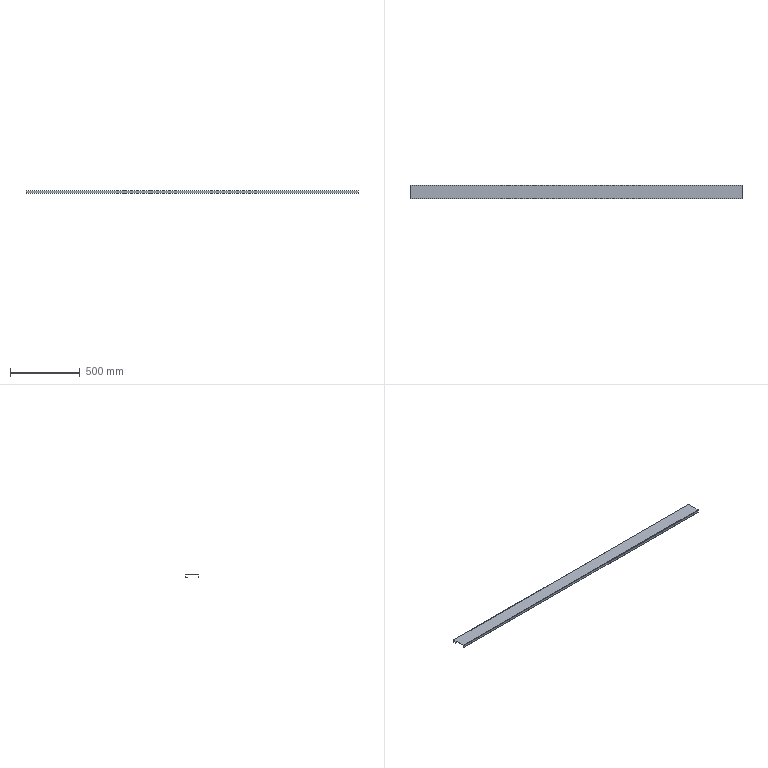Part | STEP file | E3-中转釜护栏4踢脚Plate | 1 solid | 18 faces | box 2388 x 100 x 20 mm | volume 548930 mm3 | plane 12 | cylinder 6 | commonest cylinder face diameters 2 x3 5 x3
STEP:
#1=CARTESIAN_POINT('',(0.,0.,0.));
#2=DIRECTION('',(0.,0.,1.));
#3=DIRECTION('',(1.,0.,0.));
#4=AXIS2_PLACEMENT_3D('',#1,#2,#3);
#5=CARTESIAN_POINT('',(-1194.,1.5,-2.5));
#6=VERTEX_POINT('',#5);
#7=CARTESIAN_POINT('',(-1194.,1.5,-20.));
#8=VERTEX_POINT('',#7);
#9=CARTESIAN_POINT('',(-1194.,1.5,-2.5));
#10=DIRECTION('',(0.,0.,-1.));
#11=VECTOR('',#10,1.);
#12=LINE('',#9,#11);
#13=CARTESIAN_POINT('',(1194.,1.5,-2.5));
#14=DIRECTION('',(0.,-1.,0.));
#15=DIRECTION('',(0.,0.,1.));
#16=AXIS2_PLACEMENT_3D('',#13,#14,#15);
#17=PLANE('',#16);
#18=CARTESIAN_POINT('',(0.,2388.));
#19=DIRECTION('',(-1.,0.));
#20=VECTOR('',#19,1.);
#21=LINE('',#18,#20);
#22=(GEOMETRIC_REPRESENTATION_CONTEXT(2)PARAMETRIC_REPRESENTATION_CONTEXT()REPRESENTATION_CONTEXT('',''));
#23=DEFINITIONAL_REPRESENTATION('',(#21),#22);
#24=PCURVE('',#17,#23);
#25=CARTESIAN_POINT('',(-1194.,2.5,-2.5));
#26=DIRECTION('',(-1.,0.,0.));
#27=DIRECTION('',(0.,0.,-1.));
#28=AXIS2_PLACEMENT_3D('',#25,#26,#27);
#29=PLANE('',#28);
#30=CARTESIAN_POINT('',(0.,1.));
#31=DIRECTION('',(1.,0.));
#32=VECTOR('',#31,1.);
#33=LINE('',#30,#32);
#34=(GEOMETRIC_REPRESENTATION_CONTEXT(2)PARAMETRIC_REPRESENTATION_CONTEXT()REPRESENTATION_CONTEXT('',''));
#35=DEFINITIONAL_REPRESENTATION('',(#33),#34);
#36=PCURVE('',#29,#35);
#37=SURFACE_CURVE('',#12,(#24,#36),.PCURVE_S1.);
#38=EDGE_CURVE('',#6,#8,#37,.T.);
#39=ORIENTED_EDGE('',*,*,#38,.F.);
#40=CARTESIAN_POINT('',(1194.,1.5,-2.5));
#41=VERTEX_POINT('',#40);
#42=CARTESIAN_POINT('',(1194.,1.5,-2.5));
#43=DIRECTION('',(-1.,0.,0.));
#44=VECTOR('',#43,1.);
#45=LINE('',#42,#44);
#46=CARTESIAN_POINT('',(0.,0.));
#47=DIRECTION('',(0.,1.));
#48=VECTOR('',#47,1.);
#49=LINE('',#46,#48);
#50=(GEOMETRIC_REPRESENTATION_CONTEXT(2)PARAMETRIC_REPRESENTATION_CONTEXT()REPRESENTATION_CONTEXT('',''));
#51=DEFINITIONAL_REPRESENTATION('',(#49),#50);
#52=PCURVE('',#17,#51);
#53=CARTESIAN_POINT('',(1194.,2.5,-2.5));
#54=DIRECTION('',(-1.,0.,0.));
#55=DIRECTION('',(0.,0.,-1.));
#56=AXIS2_PLACEMENT_3D('',#53,#54,#55);
#57=CYLINDRICAL_SURFACE('',#56,1.);
#58=CARTESIAN_POINT('',(1.571,0.));
#59=DIRECTION('',(0.,1.));
#60=VECTOR('',#59,1.);
#61=LINE('',#58,#60);
#62=(GEOMETRIC_REPRESENTATION_CONTEXT(2)PARAMETRIC_REPRESENTATION_CONTEXT()REPRESENTATION_CONTEXT('',''));
#63=DEFINITIONAL_REPRESENTATION('',(#61),#62);
#64=PCURVE('',#57,#63);
#65=SURFACE_CURVE('',#45,(#52,#64),.PCURVE_S1.);
#66=EDGE_CURVE('',#41,#6,#65,.T.);
#67=ORIENTED_EDGE('',*,*,#66,.F.);
#68=CARTESIAN_POINT('',(1194.,1.5,-20.));
#69=VERTEX_POINT('',#68);
#70=CARTESIAN_POINT('',(1194.,1.5,-2.5));
#71=DIRECTION('',(0.,0.,-1.));
#72=VECTOR('',#71,1.);
#73=LINE('',#70,#72);
#74=CARTESIAN_POINT('',(0.,0.));
#75=DIRECTION('',(-1.,0.));
#76=VECTOR('',#75,1.);
#77=LINE('',#74,#76);
#78=(GEOMETRIC_REPRESENTATION_CONTEXT(2)PARAMETRIC_REPRESENTATION_CONTEXT()REPRESENTATION_CONTEXT('',''));
#79=DEFINITIONAL_REPRESENTATION('',(#77),#78);
#80=PCURVE('',#17,#79);
#81=CARTESIAN_POINT('',(1194.,2.5,-2.5));
#82=DIRECTION('',(-1.,0.,0.));
#83=DIRECTION('',(0.,0.,-1.));
#84=AXIS2_PLACEMENT_3D('',#81,#82,#83);
#85=PLANE('',#84);
#86=CARTESIAN_POINT('',(0.,1.));
#87=DIRECTION('',(1.,0.));
#88=VECTOR('',#87,1.);
#89=LINE('',#86,#88);
#90=(GEOMETRIC_REPRESENTATION_CONTEXT(2)PARAMETRIC_REPRESENTATION_CONTEXT()REPRESENTATION_CONTEXT('',''));
#91=DEFINITIONAL_REPRESENTATION('',(#89),#90);
#92=PCURVE('',#85,#91);
#93=SURFACE_CURVE('',#73,(#80,#92),.PCURVE_S1.);
#94=EDGE_CURVE('',#41,#69,#93,.T.);
#95=ORIENTED_EDGE('',*,*,#94,.T.);
#96=CARTESIAN_POINT('',(1194.,1.5,-20.));
#97=DIRECTION('',(-1.,0.,0.));
#98=VECTOR('',#97,1.);
#99=LINE('',#96,#98);
#100=CARTESIAN_POINT('',(-17.5,0.));
#101=DIRECTION('',(0.,1.));
#102=VECTOR('',#101,1.);
#103=LINE('',#100,#102);
#104=(GEOMETRIC_REPRESENTATION_CONTEXT(2)PARAMETRIC_REPRESENTATION_CONTEXT()REPRESENTATION_CONTEXT('',''));
#105=DEFINITIONAL_REPRESENTATION('',(#103),#104);
#106=PCURVE('',#17,#105);
#107=CARTESIAN_POINT('',(1194.,0.,-20.));
#108=DIRECTION('',(0.,0.,-1.));
#109=DIRECTION('',(1.,0.,0.));
#110=AXIS2_PLACEMENT_3D('',#107,#108,#109);
#111=PLANE('',#110);
#112=CARTESIAN_POINT('',(0.,-1.5));
#113=DIRECTION('',(-1.,0.));
#114=VECTOR('',#113,1.);
#115=LINE('',#112,#114);
#116=(GEOMETRIC_REPRESENTATION_CONTEXT(2)PARAMETRIC_REPRESENTATION_CONTEXT()REPRESENTATION_CONTEXT('',''));
#117=DEFINITIONAL_REPRESENTATION('',(#115),#116);
#118=PCURVE('',#111,#117);
#119=SURFACE_CURVE('',#99,(#106,#118),.PCURVE_S1.);
#120=EDGE_CURVE('',#69,#8,#119,.T.);
#121=ORIENTED_EDGE('',*,*,#120,.T.);
#122=EDGE_LOOP('',(#39,#67,#95,#121));
#123=FACE_BOUND('',#122,.T.);
#124=ADVANCED_FACE('',(#123),#17,.F.);
#125=CARTESIAN_POINT('',(-1194.,0.,-20.));
#126=VERTEX_POINT('',#125);
#127=CARTESIAN_POINT('',(-1194.,0.,-20.));
#128=DIRECTION('',(0.,1.,0.));
#129=VECTOR('',#128,1.);
#130=LINE('',#127,#129);
#131=CARTESIAN_POINT('',(-2388.,0.));
#132=DIRECTION('',(0.,-1.));
#133=VECTOR('',#132,1.);
#134=LINE('',#131,#133);
#135=(GEOMETRIC_REPRESENTATION_CONTEXT(2)PARAMETRIC_REPRESENTATION_CONTEXT()REPRESENTATION_CONTEXT('',''));
#136=DEFINITIONAL_REPRESENTATION('',(#134),#135);
#137=PCURVE('',#111,#136);
#138=CARTESIAN_POINT('',(17.5,2.5));
#139=DIRECTION('',(0.,-1.));
#140=VECTOR('',#139,1.);
#141=LINE('',#138,#140);
#142=(GEOMETRIC_REPRESENTATION_CONTEXT(2)PARAMETRIC_REPRESENTATION_CONTEXT()REPRESENTATION_CONTEXT('',''));
#143=DEFINITIONAL_REPRESENTATION('',(#141),#142);
#144=PCURVE('',#29,#143);
#145=SURFACE_CURVE('',#130,(#137,#144),.PCURVE_S1.);
#146=EDGE_CURVE('',#126,#8,#145,.T.);
#147=ORIENTED_EDGE('',*,*,#146,.T.);
#148=ORIENTED_EDGE('',*,*,#120,.F.);
#149=CARTESIAN_POINT('',(1194.,0.,-20.));
#150=VERTEX_POINT('',#149);
#151=CARTESIAN_POINT('',(1194.,0.,-20.));
#152=DIRECTION('',(0.,1.,0.));
#153=VECTOR('',#152,1.);
#154=LINE('',#151,#153);
#155=CARTESIAN_POINT('',(0.,0.));
#156=DIRECTION('',(0.,-1.));
#157=VECTOR('',#156,1.);
#158=LINE('',#155,#157);
#159=(GEOMETRIC_REPRESENTATION_CONTEXT(2)PARAMETRIC_REPRESENTATION_CONTEXT()REPRESENTATION_CONTEXT('',''));
#160=DEFINITIONAL_REPRESENTATION('',(#158),#159);
#161=PCURVE('',#111,#160);
#162=CARTESIAN_POINT('',(17.5,2.5));
#163=DIRECTION('',(0.,-1.));
#164=VECTOR('',#163,1.);
#165=LINE('',#162,#164);
#166=(GEOMETRIC_REPRESENTATION_CONTEXT(2)PARAMETRIC_REPRESENTATION_CONTEXT()REPRESENTATION_CONTEXT('',''));
#167=DEFINITIONAL_REPRESENTATION('',(#165),#166);
#168=PCURVE('',#85,#167);
#169=SURFACE_CURVE('',#154,(#161,#168),.PCURVE_S1.);
#170=EDGE_CURVE('',#150,#69,#169,.T.);
#171=ORIENTED_EDGE('',*,*,#170,.F.);
#172=CARTESIAN_POINT('',(1194.,0.,-20.));
#173=DIRECTION('',(-1.,0.,0.));
#174=VECTOR('',#173,1.);
#175=LINE('',#172,#174);
#176=CARTESIAN_POINT('',(0.,0.));
#177=DIRECTION('',(-1.,0.));
#178=VECTOR('',#177,1.);
#179=LINE('',#176,#178);
#180=(GEOMETRIC_REPRESENTATION_CONTEXT(2)PARAMETRIC_REPRESENTATION_CONTEXT()REPRESENTATION_CONTEXT('',''));
#181=DEFINITIONAL_REPRESENTATION('',(#179),#180);
#182=PCURVE('',#111,#181);
#183=CARTESIAN_POINT('',(1194.,0.,-2.5));
#184=DIRECTION('',(0.,-1.,0.));
#185=DIRECTION('',(0.,0.,1.));
#186=AXIS2_PLACEMENT_3D('',#183,#184,#185);
#187=PLANE('',#186);
#188=CARTESIAN_POINT('',(-17.5,0.));
#189=DIRECTION('',(0.,1.));
#190=VECTOR('',#189,1.);
#191=LINE('',#188,#190);
#192=(GEOMETRIC_REPRESENTATION_CONTEXT(2)PARAMETRIC_REPRESENTATION_CONTEXT()REPRESENTATION_CONTEXT('',''));
#193=DEFINITIONAL_REPRESENTATION('',(#191),#192);
#194=PCURVE('',#187,#193);
#195=SURFACE_CURVE('',#175,(#182,#194),.PCURVE_S1.);
#196=EDGE_CURVE('',#150,#126,#195,.T.);
#197=ORIENTED_EDGE('',*,*,#196,.T.);
#198=EDGE_LOOP('',(#147,#148,#171,#197));
#199=FACE_BOUND('',#198,.T.);
#200=ADVANCED_FACE('',(#199),#111,.T.);
#201=CARTESIAN_POINT('',(-1194.,0.,-2.5));
#202=VERTEX_POINT('',#201);
#203=CARTESIAN_POINT('',(-1194.,0.,-2.5));
#204=DIRECTION('',(0.,0.,-1.));
#205=VECTOR('',#204,1.);
#206=LINE('',#203,#205);
#207=CARTESIAN_POINT('',(0.,2388.));
#208=DIRECTION('',(-1.,0.));
#209=VECTOR('',#208,1.);
#210=LINE('',#207,#209);
#211=(GEOMETRIC_REPRESENTATION_CONTEXT(2)PARAMETRIC_REPRESENTATION_CONTEXT()REPRESENTATION_CONTEXT('',''));
#212=DEFINITIONAL_REPRESENTATION('',(#210),#211);
#213=PCURVE('',#187,#212);
#214=CARTESIAN_POINT('',(0.,2.5));
#215=DIRECTION('',(1.,0.));
#216=VECTOR('',#215,1.);
#217=LINE('',#214,#216);
#218=(GEOMETRIC_REPRESENTATION_CONTEXT(2)PARAMETRIC_REPRESENTATION_CONTEXT()REPRESENTATION_CONTEXT('',''));
#219=DEFINITIONAL_REPRESENTATION('',(#217),#218);
#220=PCURVE('',#29,#219);
#221=SURFACE_CURVE('',#206,(#213,#220),.PCURVE_S1.);
#222=EDGE_CURVE('',#202,#126,#221,.T.);
#223=ORIENTED_EDGE('',*,*,#222,.T.);
#224=ORIENTED_EDGE('',*,*,#196,.F.);
#225=CARTESIAN_POINT('',(1194.,0.,-2.5));
#226=VERTEX_POINT('',#225);
#227=CARTESIAN_POINT('',(1194.,0.,-2.5));
#228=DIRECTION('',(0.,0.,-1.));
#229=VECTOR('',#228,1.);
#230=LINE('',#227,#229);
#231=CARTESIAN_POINT('',(0.,0.));
#232=DIRECTION('',(-1.,0.));
#233=VECTOR('',#232,1.);
#234=LINE('',#231,#233);
#235=(GEOMETRIC_REPRESENTATION_CONTEXT(2)PARAMETRIC_REPRESENTATION_CONTEXT()REPRESENTATION_CONTEXT('',''));
#236=DEFINITIONAL_REPRESENTATION('',(#234),#235);
#237=PCURVE('',#187,#236);
#238=CARTESIAN_POINT('',(0.,2.5));
#239=DIRECTION('',(1.,0.));
#240=VECTOR('',#239,1.);
#241=LINE('',#238,#240);
#242=(GEOMETRIC_REPRESENTATION_CONTEXT(2)PARAMETRIC_REPRESENTATION_CONTEXT()REPRESENTATION_CONTEXT('',''));
#243=DEFINITIONAL_REPRESENTATION('',(#241),#242);
#244=PCURVE('',#85,#243);
#245=SURFACE_CURVE('',#230,(#237,#244),.PCURVE_S1.);
#246=EDGE_CURVE('',#226,#150,#245,.T.);
#247=ORIENTED_EDGE('',*,*,#246,.F.);
#248=CARTESIAN_POINT('',(1194.,0.,-2.5));
#249=DIRECTION('',(-1.,0.,0.));
#250=VECTOR('',#249,1.);
#251=LINE('',#248,#250);
#252=CARTESIAN_POINT('',(0.,0.));
#253=DIRECTION('',(0.,1.));
#254=VECTOR('',#253,1.);
#255=LINE('',#252,#254);
#256=(GEOMETRIC_REPRESENTATION_CONTEXT(2)PARAMETRIC_REPRESENTATION_CONTEXT()REPRESENTATION_CONTEXT('',''));
#257=DEFINITIONAL_REPRESENTATION('',(#255),#256);
#258=PCURVE('',#187,#257);
#259=CARTESIAN_POINT('',(1194.,2.5,-2.5));
#260=DIRECTION('',(-1.,0.,0.));
#261=DIRECTION('',(0.,0.,-1.));
#262=AXIS2_PLACEMENT_3D('',#259,#260,#261);
#263=CYLINDRICAL_SURFACE('',#262,2.5);
#264=CARTESIAN_POINT('',(1.571,0.));
#265=DIRECTION('',(0.,1.));
#266=VECTOR('',#265,1.);
#267=LINE('',#264,#266);
#268=(GEOMETRIC_REPRESENTATION_CONTEXT(2)PARAMETRIC_REPRESENTATION_CONTEXT()REPRESENTATION_CONTEXT('',''));
#269=DEFINITIONAL_REPRESENTATION('',(#267),#268);
#270=PCURVE('',#263,#269);
#271=SURFACE_CURVE('',#251,(#258,#270),.PCURVE_S1.);
#272=EDGE_CURVE('',#226,#202,#271,.T.);
#273=ORIENTED_EDGE('',*,*,#272,.T.);
#274=EDGE_LOOP('',(#223,#224,#247,#273));
#275=FACE_BOUND('',#274,.T.);
#276=ADVANCED_FACE('',(#275),#187,.T.);
#277=CARTESIAN_POINT('',(-1194.,2.5,0.));
#278=VERTEX_POINT('',#277);
#279=CARTESIAN_POINT('',(-1194.,2.5,-2.5));
#280=DIRECTION('',(1.,0.,0.));
#281=DIRECTION('',(0.,0.,-1.));
#282=AXIS2_PLACEMENT_3D('',#279,#280,#281);
#283=CIRCLE('',#282,2.5);
#284=CARTESIAN_POINT('',(6.283,2388.));
#285=DIRECTION('',(-1.,0.));
#286=VECTOR('',#285,1.);
#287=LINE('',#284,#286);
#288=(GEOMETRIC_REPRESENTATION_CONTEXT(2)PARAMETRIC_REPRESENTATION_CONTEXT()REPRESENTATION_CONTEXT('',''));
#289=DEFINITIONAL_REPRESENTATION('',(#287),#288);
#290=PCURVE('',#263,#289);
#291=CARTESIAN_POINT('',(2.5,0.));
#292=CARTESIAN_POINT('',(2.5,-4.33));
#293=CARTESIAN_POINT('',(-1.25,-2.165));
#294=CARTESIAN_POINT('',(-5.,0.));
#295=CARTESIAN_POINT('',(-1.25,2.165));
#296=CARTESIAN_POINT('',(2.5,4.33));
#297=CARTESIAN_POINT('',(2.5,0.));
#298=(BOUNDED_CURVE()B_SPLINE_CURVE(2,(#291,#292,#293,#294,#295,#296,#297),.UNSPECIFIED.,.T.,.F.)B_SPLINE_CURVE_WITH_KNOTS((1,2,2,2,2,1),(-2.094,0.,2.094,4.189,6.283,8.378),.UNSPECIFIED.)CURVE()GEOMETRIC_REPRESENTATION_ITEM()RATIONAL_B_SPLINE_CURVE((1.,0.5,1.,0.5,1.,0.5,1.))REPRESENTATION_ITEM(''));
#299=(GEOMETRIC_REPRESENTATION_CONTEXT(2)PARAMETRIC_REPRESENTATION_CONTEXT()REPRESENTATION_CONTEXT('',''));
#300=DEFINITIONAL_REPRESENTATION('',(#298),#299);
#301=PCURVE('',#29,#300);
#302=SURFACE_CURVE('',#283,(#290,#301),.PCURVE_S1.);
#303=EDGE_CURVE('',#278,#202,#302,.T.);
#304=ORIENTED_EDGE('',*,*,#303,.T.);
#305=ORIENTED_EDGE('',*,*,#272,.F.);
#306=CARTESIAN_POINT('',(1194.,2.5,0.));
#307=VERTEX_POINT('',#306);
#308=CARTESIAN_POINT('',(1194.,2.5,-2.5));
#309=DIRECTION('',(1.,0.,0.));
#310=DIRECTION('',(0.,0.,-1.));
#311=AXIS2_PLACEMENT_3D('',#308,#309,#310);
#312=CIRCLE('',#311,2.5);
#313=CARTESIAN_POINT('',(6.283,0.));
#314=DIRECTION('',(-1.,0.));
#315=VECTOR('',#314,1.);
#316=LINE('',#313,#315);
#317=(GEOMETRIC_REPRESENTATION_CONTEXT(2)PARAMETRIC_REPRESENTATION_CONTEXT()REPRESENTATION_CONTEXT('',''));
#318=DEFINITIONAL_REPRESENTATION('',(#316),#317);
#319=PCURVE('',#263,#318);
#320=CARTESIAN_POINT('',(2.5,0.));
#321=CARTESIAN_POINT('',(2.5,-4.33));
#322=CARTESIAN_POINT('',(-1.25,-2.165));
#323=CARTESIAN_POINT('',(-5.,0.));
#324=CARTESIAN_POINT('',(-1.25,2.165));
#325=CARTESIAN_POINT('',(2.5,4.33));
#326=CARTESIAN_POINT('',(2.5,0.));
#327=(BOUNDED_CURVE()B_SPLINE_CURVE(2,(#320,#321,#322,#323,#324,#325,#326),.UNSPECIFIED.,.T.,.F.)B_SPLINE_CURVE_WITH_KNOTS((1,2,2,2,2,1),(-2.094,0.,2.094,4.189,6.283,8.378),.UNSPECIFIED.)CURVE()GEOMETRIC_REPRESENTATION_ITEM()RATIONAL_B_SPLINE_CURVE((1.,0.5,1.,0.5,1.,0.5,1.))REPRESENTATION_ITEM(''));
#328=(GEOMETRIC_REPRESENTATION_CONTEXT(2)PARAMETRIC_REPRESENTATION_CONTEXT()REPRESENTATION_CONTEXT('',''));
#329=DEFINITIONAL_REPRESENTATION('',(#327),#328);
#330=PCURVE('',#85,#329);
#331=SURFACE_CURVE('',#312,(#319,#330),.PCURVE_S1.);
#332=EDGE_CURVE('',#307,#226,#331,.T.);
#333=ORIENTED_EDGE('',*,*,#332,.F.);
#334=CARTESIAN_POINT('',(1194.,2.5,0.));
#335=DIRECTION('',(-1.,0.,0.));
#336=VECTOR('',#335,1.);
#337=LINE('',#334,#336);
#338=CARTESIAN_POINT('',(3.142,0.));
#339=DIRECTION('',(0.,1.));
#340=VECTOR('',#339,1.);
#341=LINE('',#338,#340);
#342=(GEOMETRIC_REPRESENTATION_CONTEXT(2)PARAMETRIC_REPRESENTATION_CONTEXT()REPRESENTATION_CONTEXT('',''));
#343=DEFINITIONAL_REPRESENTATION('',(#341),#342);
#344=PCURVE('',#263,#343);
#345=CARTESIAN_POINT('',(1194.,2.5,0.));
#346=DIRECTION('',(0.,0.,1.));
#347=DIRECTION('',(-1.,0.,0.));
#348=AXIS2_PLACEMENT_3D('',#345,#346,#347);
#349=PLANE('',#348);
#350=CARTESIAN_POINT('',(0.,0.));
#351=DIRECTION('',(1.,0.));
#352=VECTOR('',#351,1.);
#353=LINE('',#350,#352);
#354=(GEOMETRIC_REPRESENTATION_CONTEXT(2)PARAMETRIC_REPRESENTATION_CONTEXT()REPRESENTATION_CONTEXT('',''));
#355=DEFINITIONAL_REPRESENTATION('',(#353),#354);
#356=PCURVE('',#349,#355);
#357=SURFACE_CURVE('',#337,(#344,#356),.PCURVE_S1.);
#358=EDGE_CURVE('',#307,#278,#357,.T.);
#359=ORIENTED_EDGE('',*,*,#358,.T.);
#360=EDGE_LOOP('',(#304,#305,#333,#359));
#361=FACE_BOUND('',#360,.T.);
#362=ADVANCED_FACE('',(#361),#263,.T.);
#363=CARTESIAN_POINT('',(-1194.,97.5,0.));
#364=VERTEX_POINT('',#363);
#365=CARTESIAN_POINT('',(-1194.,2.5,0.));
#366=DIRECTION('',(0.,-1.,0.));
#367=VECTOR('',#366,1.);
#368=LINE('',#365,#367);
#369=CARTESIAN_POINT('',(2388.,0.));
#370=DIRECTION('',(0.,1.));
#371=VECTOR('',#370,1.);
#372=LINE('',#369,#371);
#373=(GEOMETRIC_REPRESENTATION_CONTEXT(2)PARAMETRIC_REPRESENTATION_CONTEXT()REPRESENTATION_CONTEXT('',''));
#374=DEFINITIONAL_REPRESENTATION('',(#372),#373);
#375=PCURVE('',#349,#374);
#376=CARTESIAN_POINT('',(-2.5,0.));
#377=DIRECTION('',(0.,1.));
#378=VECTOR('',#377,1.);
#379=LINE('',#376,#378);
#380=(GEOMETRIC_REPRESENTATION_CONTEXT(2)PARAMETRIC_REPRESENTATION_CONTEXT()REPRESENTATION_CONTEXT('',''));
#381=DEFINITIONAL_REPRESENTATION('',(#379),#380);
#382=PCURVE('',#29,#381);
#383=SURFACE_CURVE('',#368,(#375,#382),.PCURVE_S1.);
#384=EDGE_CURVE('',#364,#278,#383,.T.);
#385=ORIENTED_EDGE('',*,*,#384,.T.);
#386=ORIENTED_EDGE('',*,*,#358,.F.);
#387=CARTESIAN_POINT('',(1194.,97.5,0.));
#388=VERTEX_POINT('',#387);
#389=CARTESIAN_POINT('',(1194.,2.5,0.));
#390=DIRECTION('',(0.,-1.,0.));
#391=VECTOR('',#390,1.);
#392=LINE('',#389,#391);
#393=CARTESIAN_POINT('',(0.,0.));
#394=DIRECTION('',(0.,1.));
#395=VECTOR('',#394,1.);
#396=LINE('',#393,#395);
#397=(GEOMETRIC_REPRESENTATION_CONTEXT(2)PARAMETRIC_REPRESENTATION_CONTEXT()REPRESENTATION_CONTEXT('',''));
#398=DEFINITIONAL_REPRESENTATION('',(#396),#397);
#399=PCURVE('',#349,#398);
#400=CARTESIAN_POINT('',(-2.5,0.));
#401=DIRECTION('',(0.,1.));
#402=VECTOR('',#401,1.);
#403=LINE('',#400,#402);
#404=(GEOMETRIC_REPRESENTATION_CONTEXT(2)PARAMETRIC_REPRESENTATION_CONTEXT()REPRESENTATION_CONTEXT('',''));
#405=DEFINITIONAL_REPRESENTATION('',(#403),#404);
#406=PCURVE('',#85,#405);
#407=SURFACE_CURVE('',#392,(#399,#406),.PCURVE_S1.);
#408=EDGE_CURVE('',#388,#307,#407,.T.);
#409=ORIENTED_EDGE('',*,*,#408,.F.);
#410=CARTESIAN_POINT('',(1194.,97.5,0.));
#411=DIRECTION('',(-1.,0.,0.));
#412=VECTOR('',#411,1.);
#413=LINE('',#410,#412);
#414=CARTESIAN_POINT('',(0.,-95.));
#415=DIRECTION('',(1.,0.));
#416=VECTOR('',#415,1.);
#417=LINE('',#414,#416);
#418=(GEOMETRIC_REPRESENTATION_CONTEXT(2)PARAMETRIC_REPRESENTATION_CONTEXT()REPRESENTATION_CONTEXT('',''));
#419=DEFINITIONAL_REPRESENTATION('',(#417),#418);
#420=PCURVE('',#349,#419);
#421=CARTESIAN_POINT('',(1194.,97.5,-2.5));
#422=DIRECTION('',(-1.,0.,0.));
#423=DIRECTION('',(0.,0.,-1.));
#424=AXIS2_PLACEMENT_3D('',#421,#422,#423);
#425=CYLINDRICAL_SURFACE('',#424,2.5);
#426=CARTESIAN_POINT('',(3.142,0.));
#427=DIRECTION('',(0.,1.));
#428=VECTOR('',#427,1.);
#429=LINE('',#426,#428);
#430=(GEOMETRIC_REPRESENTATION_CONTEXT(2)PARAMETRIC_REPRESENTATION_CONTEXT()REPRESENTATION_CONTEXT('',''));
#431=DEFINITIONAL_REPRESENTATION('',(#429),#430);
#432=PCURVE('',#425,#431);
#433=SURFACE_CURVE('',#413,(#420,#432),.PCURVE_S1.);
#434=EDGE_CURVE('',#388,#364,#433,.T.);
#435=ORIENTED_EDGE('',*,*,#434,.T.);
#436=EDGE_LOOP('',(#385,#386,#409,#435));
#437=FACE_BOUND('',#436,.T.);
#438=ADVANCED_FACE('',(#437),#349,.T.);
#439=CARTESIAN_POINT('',(-1194.,100.,-2.5));
#440=VERTEX_POINT('',#439);
#441=CARTESIAN_POINT('',(-1194.,97.5,-2.5));
#442=DIRECTION('',(1.,0.,0.));
#443=DIRECTION('',(0.,0.,1.));
#444=AXIS2_PLACEMENT_3D('',#441,#442,#443);
#445=CIRCLE('',#444,2.5);
#446=CARTESIAN_POINT('',(9.425,2388.));
#447=DIRECTION('',(-1.,0.));
#448=VECTOR('',#447,1.);
#449=LINE('',#446,#448);
#450=(GEOMETRIC_REPRESENTATION_CONTEXT(2)PARAMETRIC_REPRESENTATION_CONTEXT()REPRESENTATION_CONTEXT('',''));
#451=DEFINITIONAL_REPRESENTATION('',(#449),#450);
#452=PCURVE('',#425,#451);
#453=CARTESIAN_POINT('',(-2.5,-95.));
#454=CARTESIAN_POINT('',(-2.5,-90.67));
#455=CARTESIAN_POINT('',(1.25,-92.835));
#456=CARTESIAN_POINT('',(5.,-95.));
#457=CARTESIAN_POINT('',(1.25,-97.165));
#458=CARTESIAN_POINT('',(-2.5,-99.33));
#459=CARTESIAN_POINT('',(-2.5,-95.));
#460=(BOUNDED_CURVE()B_SPLINE_CURVE(2,(#453,#454,#455,#456,#457,#458,#459),.UNSPECIFIED.,.T.,.F.)B_SPLINE_CURVE_WITH_KNOTS((1,2,2,2,2,1),(-2.094,0.,2.094,4.189,6.283,8.378),.UNSPECIFIED.)CURVE()GEOMETRIC_REPRESENTATION_ITEM()RATIONAL_B_SPLINE_CURVE((1.,0.5,1.,0.5,1.,0.5,1.))REPRESENTATION_ITEM(''));
#461=(GEOMETRIC_REPRESENTATION_CONTEXT(2)PARAMETRIC_REPRESENTATION_CONTEXT()REPRESENTATION_CONTEXT('',''));
#462=DEFINITIONAL_REPRESENTATION('',(#460),#461);
#463=PCURVE('',#29,#462);
#464=SURFACE_CURVE('',#445,(#452,#463),.PCURVE_S1.);
#465=EDGE_CURVE('',#440,#364,#464,.T.);
#466=ORIENTED_EDGE('',*,*,#465,.T.);
#467=ORIENTED_EDGE('',*,*,#434,.F.);
#468=CARTESIAN_POINT('',(1194.,100.,-2.5));
#469=VERTEX_POINT('',#468);
#470=CARTESIAN_POINT('',(1194.,97.5,-2.5));
#471=DIRECTION('',(1.,0.,0.));
#472=DIRECTION('',(0.,0.,1.));
#473=AXIS2_PLACEMENT_3D('',#470,#471,#472);
#474=CIRCLE('',#473,2.5);
#475=CARTESIAN_POINT('',(9.425,0.));
#476=DIRECTION('',(-1.,0.));
#477=VECTOR('',#476,1.);
#478=LINE('',#475,#477);
#479=(GEOMETRIC_REPRESENTATION_CONTEXT(2)PARAMETRIC_REPRESENTATION_CONTEXT()REPRESENTATION_CONTEXT('',''));
#480=DEFINITIONAL_REPRESENTATION('',(#478),#479);
#481=PCURVE('',#425,#480);
#482=CARTESIAN_POINT('',(-2.5,-95.));
#483=CARTESIAN_POINT('',(-2.5,-90.67));
#484=CARTESIAN_POINT('',(1.25,-92.835));
#485=CARTESIAN_POINT('',(5.,-95.));
#486=CARTESIAN_POINT('',(1.25,-97.165));
#487=CARTESIAN_POINT('',(-2.5,-99.33));
#488=CARTESIAN_POINT('',(-2.5,-95.));
#489=(BOUNDED_CURVE()B_SPLINE_CURVE(2,(#482,#483,#484,#485,#486,#487,#488),.UNSPECIFIED.,.T.,.F.)B_SPLINE_CURVE_WITH_KNOTS((1,2,2,2,2,1),(-2.094,0.,2.094,4.189,6.283,8.378),.UNSPECIFIED.)CURVE()GEOMETRIC_REPRESENTATION_ITEM()RATIONAL_B_SPLINE_CURVE((1.,0.5,1.,0.5,1.,0.5,1.))REPRESENTATION_ITEM(''));
#490=(GEOMETRIC_REPRESENTATION_CONTEXT(2)PARAMETRIC_REPRESENTATION_CONTEXT()REPRESENTATION_CONTEXT('',''));
#491=DEFINITIONAL_REPRESENTATION('',(#489),#490);
#492=PCURVE('',#85,#491);
#493=SURFACE_CURVE('',#474,(#481,#492),.PCURVE_S1.);
#494=EDGE_CURVE('',#469,#388,#493,.T.);
#495=ORIENTED_EDGE('',*,*,#494,.F.);
#496=CARTESIAN_POINT('',(1194.,100.,-2.5));
#497=DIRECTION('',(-1.,0.,0.));
#498=VECTOR('',#497,1.);
#499=LINE('',#496,#498);
#500=CARTESIAN_POINT('',(4.712,0.));
#501=DIRECTION('',(0.,1.));
#502=VECTOR('',#501,1.);
#503=LINE('',#500,#502);
#504=(GEOMETRIC_REPRESENTATION_CONTEXT(2)PARAMETRIC_REPRESENTATION_CONTEXT()REPRESENTATION_CONTEXT('',''));
#505=DEFINITIONAL_REPRESENTATION('',(#503),#504);
#506=PCURVE('',#425,#505);
#507=CARTESIAN_POINT('',(1194.,100.,-2.5));
#508=DIRECTION('',(0.,1.,0.));
#509=DIRECTION('',(0.,0.,-1.));
#510=AXIS2_PLACEMENT_3D('',#507,#508,#509);
#511=PLANE('',#510);
#512=CARTESIAN_POINT('',(0.,0.));
#513=DIRECTION('',(0.,1.));
#514=VECTOR('',#513,1.);
#515=LINE('',#512,#514);
#516=(GEOMETRIC_REPRESENTATION_CONTEXT(2)PARAMETRIC_REPRESENTATION_CONTEXT()REPRESENTATION_CONTEXT('',''));
#517=DEFINITIONAL_REPRESENTATION('',(#515),#516);
#518=PCURVE('',#511,#517);
#519=SURFACE_CURVE('',#499,(#506,#518),.PCURVE_S1.);
#520=EDGE_CURVE('',#469,#440,#519,.T.);
#521=ORIENTED_EDGE('',*,*,#520,.T.);
#522=EDGE_LOOP('',(#466,#467,#495,#521));
#523=FACE_BOUND('',#522,.T.);
#524=ADVANCED_FACE('',(#523),#425,.T.);
#525=CARTESIAN_POINT('',(-1194.,100.,-17.5));
#526=VERTEX_POINT('',#525);
#527=CARTESIAN_POINT('',(-1194.,100.,-2.5));
#528=DIRECTION('',(0.,0.,1.));
#529=VECTOR('',#528,1.);
#530=LINE('',#527,#529);
#531=CARTESIAN_POINT('',(0.,2388.));
#532=DIRECTION('',(-1.,0.));
#533=VECTOR('',#532,1.);
#534=LINE('',#531,#533);
#535=(GEOMETRIC_REPRESENTATION_CONTEXT(2)PARAMETRIC_REPRESENTATION_CONTEXT()REPRESENTATION_CONTEXT('',''));
#536=DEFINITIONAL_REPRESENTATION('',(#534),#535);
#537=PCURVE('',#511,#536);
#538=CARTESIAN_POINT('',(0.,-97.5));
#539=DIRECTION('',(-1.,0.));
#540=VECTOR('',#539,1.);
#541=LINE('',#538,#540);
#542=(GEOMETRIC_REPRESENTATION_CONTEXT(2)PARAMETRIC_REPRESENTATION_CONTEXT()REPRESENTATION_CONTEXT('',''));
#543=DEFINITIONAL_REPRESENTATION('',(#541),#542);
#544=PCURVE('',#29,#543);
#545=SURFACE_CURVE('',#530,(#537,#544),.PCURVE_S1.);
#546=EDGE_CURVE('',#526,#440,#545,.T.);
#547=ORIENTED_EDGE('',*,*,#546,.T.);
#548=ORIENTED_EDGE('',*,*,#520,.F.);
#549=CARTESIAN_POINT('',(1194.,100.,-17.5));
#550=VERTEX_POINT('',#549);
#551=CARTESIAN_POINT('',(1194.,100.,-2.5));
#552=DIRECTION('',(0.,0.,1.));
#553=VECTOR('',#552,1.);
#554=LINE('',#551,#553);
#555=CARTESIAN_POINT('',(0.,0.));
#556=DIRECTION('',(-1.,0.));
#557=VECTOR('',#556,1.);
#558=LINE('',#555,#557);
#559=(GEOMETRIC_REPRESENTATION_CONTEXT(2)PARAMETRIC_REPRESENTATION_CONTEXT()REPRESENTATION_CONTEXT('',''));
#560=DEFINITIONAL_REPRESENTATION('',(#558),#559);
#561=PCURVE('',#511,#560);
#562=CARTESIAN_POINT('',(0.,-97.5));
#563=DIRECTION('',(-1.,0.));
#564=VECTOR('',#563,1.);
#565=LINE('',#562,#564);
#566=(GEOMETRIC_REPRESENTATION_CONTEXT(2)PARAMETRIC_REPRESENTATION_CONTEXT()REPRESENTATION_CONTEXT('',''));
#567=DEFINITIONAL_REPRESENTATION('',(#565),#566);
#568=PCURVE('',#85,#567);
#569=SURFACE_CURVE('',#554,(#561,#568),.PCURVE_S1.);
#570=EDGE_CURVE('',#550,#469,#569,.T.);
#571=ORIENTED_EDGE('',*,*,#570,.F.);
#572=CARTESIAN_POINT('',(1194.,100.,-17.5));
#573=DIRECTION('',(-1.,0.,0.));
#574=VECTOR('',#573,1.);
#575=LINE('',#572,#574);
#576=CARTESIAN_POINT('',(15.,0.));
#577=DIRECTION('',(0.,1.));
#578=VECTOR('',#577,1.);
#579=LINE('',#576,#578);
#580=(GEOMETRIC_REPRESENTATION_CONTEXT(2)PARAMETRIC_REPRESENTATION_CONTEXT()REPRESENTATION_CONTEXT('',''));
#581=DEFINITIONAL_REPRESENTATION('',(#579),#580);
#582=PCURVE('',#511,#581);
#583=CARTESIAN_POINT('',(1194.,97.5,-17.5));
#584=DIRECTION('',(-1.,0.,0.));
#585=DIRECTION('',(0.,0.,-1.));
#586=AXIS2_PLACEMENT_3D('',#583,#584,#585);
#587=CYLINDRICAL_SURFACE('',#586,2.5);
#588=CARTESIAN_POINT('',(4.712,0.));
#589=DIRECTION('',(0.,1.));
#590=VECTOR('',#589,1.);
#591=LINE('',#588,#590);
#592=(GEOMETRIC_REPRESENTATION_CONTEXT(2)PARAMETRIC_REPRESENTATION_CONTEXT()REPRESENTATION_CONTEXT('',''));
#593=DEFINITIONAL_REPRESENTATION('',(#591),#592);
#594=PCURVE('',#587,#593);
#595=SURFACE_CURVE('',#575,(#582,#594),.PCURVE_S1.);
#596=EDGE_CURVE('',#550,#526,#595,.T.);
#597=ORIENTED_EDGE('',*,*,#596,.T.);
#598=EDGE_LOOP('',(#547,#548,#571,#597));
#599=FACE_BOUND('',#598,.T.);
#600=ADVANCED_FACE('',(#599),#511,.T.);
#601=CARTESIAN_POINT('',(-1194.,97.5,-20.));
#602=VERTEX_POINT('',#601);
#603=CARTESIAN_POINT('',(-1194.,97.5,-17.5));
#604=DIRECTION('',(1.,0.,0.));
#605=DIRECTION('',(0.,0.,1.));
#606=AXIS2_PLACEMENT_3D('',#603,#604,#605);
#607=CIRCLE('',#606,2.5);
#608=CARTESIAN_POINT('',(9.425,2388.));
#609=DIRECTION('',(-1.,0.));
#610=VECTOR('',#609,1.);
#611=LINE('',#608,#610);
#612=(GEOMETRIC_REPRESENTATION_CONTEXT(2)PARAMETRIC_REPRESENTATION_CONTEXT()REPRESENTATION_CONTEXT('',''));
#613=DEFINITIONAL_REPRESENTATION('',(#611),#612);
#614=PCURVE('',#587,#613);
#615=CARTESIAN_POINT('',(12.5,-95.));
#616=CARTESIAN_POINT('',(12.5,-90.67));
#617=CARTESIAN_POINT('',(16.25,-92.835));
#618=CARTESIAN_POINT('',(20.,-95.));
#619=CARTESIAN_POINT('',(16.25,-97.165));
#620=CARTESIAN_POINT('',(12.5,-99.33));
#621=CARTESIAN_POINT('',(12.5,-95.));
#622=(BOUNDED_CURVE()B_SPLINE_CURVE(2,(#615,#616,#617,#618,#619,#620,#621),.UNSPECIFIED.,.T.,.F.)B_SPLINE_CURVE_WITH_KNOTS((1,2,2,2,2,1),(-2.094,0.,2.094,4.189,6.283,8.378),.UNSPECIFIED.)CURVE()GEOMETRIC_REPRESENTATION_ITEM()RATIONAL_B_SPLINE_CURVE((1.,0.5,1.,0.5,1.,0.5,1.))REPRESENTATION_ITEM(''));
#623=(GEOMETRIC_REPRESENTATION_CONTEXT(2)PARAMETRIC_REPRESENTATION_CONTEXT()REPRESENTATION_CONTEXT('',''));
#624=DEFINITIONAL_REPRESENTATION('',(#622),#623);
#625=PCURVE('',#29,#624);
#626=SURFACE_CURVE('',#607,(#614,#625),.PCURVE_S1.);
#627=EDGE_CURVE('',#602,#526,#626,.T.);
#628=ORIENTED_EDGE('',*,*,#627,.T.);
#629=ORIENTED_EDGE('',*,*,#596,.F.);
#630=CARTESIAN_POINT('',(1194.,97.5,-20.));
#631=VERTEX_POINT('',#630);
#632=CARTESIAN_POINT('',(1194.,97.5,-17.5));
#633=DIRECTION('',(1.,0.,0.));
#634=DIRECTION('',(0.,0.,1.));
#635=AXIS2_PLACEMENT_3D('',#632,#633,#634);
#636=CIRCLE('',#635,2.5);
#637=CARTESIAN_POINT('',(9.425,0.));
#638=DIRECTION('',(-1.,0.));
#639=VECTOR('',#638,1.);
#640=LINE('',#637,#639);
#641=(GEOMETRIC_REPRESENTATION_CONTEXT(2)PARAMETRIC_REPRESENTATION_CONTEXT()REPRESENTATION_CONTEXT('',''));
#642=DEFINITIONAL_REPRESENTATION('',(#640),#641);
#643=PCURVE('',#587,#642);
#644=CARTESIAN_POINT('',(12.5,-95.));
#645=CARTESIAN_POINT('',(12.5,-90.67));
#646=CARTESIAN_POINT('',(16.25,-92.835));
#647=CARTESIAN_POINT('',(20.,-95.));
#648=CARTESIAN_POINT('',(16.25,-97.165));
#649=CARTESIAN_POINT('',(12.5,-99.33));
#650=CARTESIAN_POINT('',(12.5,-95.));
#651=(BOUNDED_CURVE()B_SPLINE_CURVE(2,(#644,#645,#646,#647,#648,#649,#650),.UNSPECIFIED.,.T.,.F.)B_SPLINE_CURVE_WITH_KNOTS((1,2,2,2,2,1),(-2.094,0.,2.094,4.189,6.283,8.378),.UNSPECIFIED.)CURVE()GEOMETRIC_REPRESENTATION_ITEM()RATIONAL_B_SPLINE_CURVE((1.,0.5,1.,0.5,1.,0.5,1.))REPRESENTATION_ITEM(''));
#652=(GEOMETRIC_REPRESENTATION_CONTEXT(2)PARAMETRIC_REPRESENTATION_CONTEXT()REPRESENTATION_CONTEXT('',''));
#653=DEFINITIONAL_REPRESENTATION('',(#651),#652);
#654=PCURVE('',#85,#653);
#655=SURFACE_CURVE('',#636,(#643,#654),.PCURVE_S1.);
#656=EDGE_CURVE('',#631,#550,#655,.T.);
#657=ORIENTED_EDGE('',*,*,#656,.F.);
#658=CARTESIAN_POINT('',(1194.,97.5,-20.));
#659=DIRECTION('',(-1.,0.,0.));
#660=VECTOR('',#659,1.);
#661=LINE('',#658,#660);
#662=CARTESIAN_POINT('',(6.283,0.));
#663=DIRECTION('',(0.,1.));
#664=VECTOR('',#663,1.);
#665=LINE('',#662,#664);
#666=(GEOMETRIC_REPRESENTATION_CONTEXT(2)PARAMETRIC_REPRESENTATION_CONTEXT()REPRESENTATION_CONTEXT('',''));
#667=DEFINITIONAL_REPRESENTATION('',(#665),#666);
#668=PCURVE('',#587,#667);
#669=CARTESIAN_POINT('',(1194.,97.5,-20.));
#670=DIRECTION('',(0.,0.,-1.));
#671=DIRECTION('',(1.,0.,0.));
#672=AXIS2_PLACEMENT_3D('',#669,#670,#671);
#673=PLANE('',#672);
#674=CARTESIAN_POINT('',(0.,0.));
#675=DIRECTION('',(-1.,0.));
#676=VECTOR('',#675,1.);
#677=LINE('',#674,#676);
#678=(GEOMETRIC_REPRESENTATION_CONTEXT(2)PARAMETRIC_REPRESENTATION_CONTEXT()REPRESENTATION_CONTEXT('',''));
#679=DEFINITIONAL_REPRESENTATION('',(#677),#678);
#680=PCURVE('',#673,#679);
#681=SURFACE_CURVE('',#661,(#668,#680),.PCURVE_S1.);
#682=EDGE_CURVE('',#631,#602,#681,.T.);
#683=ORIENTED_EDGE('',*,*,#682,.T.);
#684=EDGE_LOOP('',(#628,#629,#657,#683));
#685=FACE_BOUND('',#684,.T.);
#686=ADVANCED_FACE('',(#685),#587,.T.);
#687=CARTESIAN_POINT('',(-1194.,80.,-20.));
#688=VERTEX_POINT('',#687);
#689=CARTESIAN_POINT('',(-1194.,97.5,-20.));
#690=DIRECTION('',(0.,1.,0.));
#691=VECTOR('',#690,1.);
#692=LINE('',#689,#691);
#693=CARTESIAN_POINT('',(-2388.,0.));
#694=DIRECTION('',(0.,-1.));
#695=VECTOR('',#694,1.);
#696=LINE('',#693,#695);
#697=(GEOMETRIC_REPRESENTATION_CONTEXT(2)PARAMETRIC_REPRESENTATION_CONTEXT()REPRESENTATION_CONTEXT('',''));
#698=DEFINITIONAL_REPRESENTATION('',(#696),#697);
#699=PCURVE('',#673,#698);
#700=CARTESIAN_POINT('',(17.5,-95.));
#701=DIRECTION('',(0.,-1.));
#702=VECTOR('',#701,1.);
#703=LINE('',#700,#702);
#704=(GEOMETRIC_REPRESENTATION_CONTEXT(2)PARAMETRIC_REPRESENTATION_CONTEXT()REPRESENTATION_CONTEXT('',''));
#705=DEFINITIONAL_REPRESENTATION('',(#703),#704);
#706=PCURVE('',#29,#705);
#707=SURFACE_CURVE('',#692,(#699,#706),.PCURVE_S1.);
#708=EDGE_CURVE('',#688,#602,#707,.T.);
#709=ORIENTED_EDGE('',*,*,#708,.T.);
#710=ORIENTED_EDGE('',*,*,#682,.F.);
#711=CARTESIAN_POINT('',(1194.,80.,-20.));
#712=VERTEX_POINT('',#711);
#713=CARTESIAN_POINT('',(1194.,97.5,-20.));
#714=DIRECTION('',(0.,1.,0.));
#715=VECTOR('',#714,1.);
#716=LINE('',#713,#715);
#717=CARTESIAN_POINT('',(0.,0.));
#718=DIRECTION('',(0.,-1.));
#719=VECTOR('',#718,1.);
#720=LINE('',#717,#719);
#721=(GEOMETRIC_REPRESENTATION_CONTEXT(2)PARAMETRIC_REPRESENTATION_CONTEXT()REPRESENTATION_CONTEXT('',''));
#722=DEFINITIONAL_REPRESENTATION('',(#720),#721);
#723=PCURVE('',#673,#722);
#724=CARTESIAN_POINT('',(17.5,-95.));
#725=DIRECTION('',(0.,-1.));
#726=VECTOR('',#725,1.);
#727=LINE('',#724,#726);
#728=(GEOMETRIC_REPRESENTATION_CONTEXT(2)PARAMETRIC_REPRESENTATION_CONTEXT()REPRESENTATION_CONTEXT('',''));
#729=DEFINITIONAL_REPRESENTATION('',(#727),#728);
#730=PCURVE('',#85,#729);
#731=SURFACE_CURVE('',#716,(#723,#730),.PCURVE_S1.);
#732=EDGE_CURVE('',#712,#631,#731,.T.);
#733=ORIENTED_EDGE('',*,*,#732,.F.);
#734=CARTESIAN_POINT('',(1194.,80.,-20.));
#735=DIRECTION('',(-1.,0.,0.));
#736=VECTOR('',#735,1.);
#737=LINE('',#734,#736);
#738=CARTESIAN_POINT('',(0.,17.5));
#739=DIRECTION('',(-1.,0.));
#740=VECTOR('',#739,1.);
#741=LINE('',#738,#740);
#742=(GEOMETRIC_REPRESENTATION_CONTEXT(2)PARAMETRIC_REPRESENTATION_CONTEXT()REPRESENTATION_CONTEXT('',''));
#743=DEFINITIONAL_REPRESENTATION('',(#741),#742);
#744=PCURVE('',#673,#743);
#745=CARTESIAN_POINT('',(1194.,80.,-18.5));
#746=DIRECTION('',(0.,-1.,0.));
#747=DIRECTION('',(0.,0.,1.));
#748=AXIS2_PLACEMENT_3D('',#745,#746,#747);
#749=PLANE('',#748);
#750=CARTESIAN_POINT('',(-1.5,0.));
#751=DIRECTION('',(0.,1.));
#752=VECTOR('',#751,1.);
#753=LINE('',#750,#752);
#754=(GEOMETRIC_REPRESENTATION_CONTEXT(2)PARAMETRIC_REPRESENTATION_CONTEXT()REPRESENTATION_CONTEXT('',''));
#755=DEFINITIONAL_REPRESENTATION('',(#753),#754);
#756=PCURVE('',#749,#755);
#757=SURFACE_CURVE('',#737,(#744,#756),.PCURVE_S1.);
#758=EDGE_CURVE('',#712,#688,#757,.T.);
#759=ORIENTED_EDGE('',*,*,#758,.T.);
#760=EDGE_LOOP('',(#709,#710,#733,#759));
#761=FACE_BOUND('',#760,.T.);
#762=ADVANCED_FACE('',(#761),#673,.T.);
#763=CARTESIAN_POINT('',(-1194.,80.,-18.5));
#764=VERTEX_POINT('',#763);
#765=CARTESIAN_POINT('',(-1194.,80.,-18.5));
#766=DIRECTION('',(0.,0.,-1.));
#767=VECTOR('',#766,1.);
#768=LINE('',#765,#767);
#769=CARTESIAN_POINT('',(0.,2388.));
#770=DIRECTION('',(-1.,0.));
#771=VECTOR('',#770,1.);
#772=LINE('',#769,#771);
#773=(GEOMETRIC_REPRESENTATION_CONTEXT(2)PARAMETRIC_REPRESENTATION_CONTEXT()REPRESENTATION_CONTEXT('',''));
#774=DEFINITIONAL_REPRESENTATION('',(#772),#773);
#775=PCURVE('',#749,#774);
#776=CARTESIAN_POINT('',(16.,-77.5));
#777=DIRECTION('',(1.,0.));
#778=VECTOR('',#777,1.);
#779=LINE('',#776,#778);
#780=(GEOMETRIC_REPRESENTATION_CONTEXT(2)PARAMETRIC_REPRESENTATION_CONTEXT()REPRESENTATION_CONTEXT('',''));
#781=DEFINITIONAL_REPRESENTATION('',(#779),#780);
#782=PCURVE('',#29,#781);
#783=SURFACE_CURVE('',#768,(#775,#782),.PCURVE_S1.);
#784=EDGE_CURVE('',#764,#688,#783,.T.);
#785=ORIENTED_EDGE('',*,*,#784,.T.);
#786=ORIENTED_EDGE('',*,*,#758,.F.);
#787=CARTESIAN_POINT('',(1194.,80.,-18.5));
#788=VERTEX_POINT('',#787);
#789=CARTESIAN_POINT('',(1194.,80.,-18.5));
#790=DIRECTION('',(0.,0.,-1.));
#791=VECTOR('',#790,1.);
#792=LINE('',#789,#791);
#793=CARTESIAN_POINT('',(0.,0.));
#794=DIRECTION('',(-1.,0.));
#795=VECTOR('',#794,1.);
#796=LINE('',#793,#795);
#797=(GEOMETRIC_REPRESENTATION_CONTEXT(2)PARAMETRIC_REPRESENTATION_CONTEXT()REPRESENTATION_CONTEXT('',''));
#798=DEFINITIONAL_REPRESENTATION('',(#796),#797);
#799=PCURVE('',#749,#798);
#800=CARTESIAN_POINT('',(16.,-77.5));
#801=DIRECTION('',(1.,0.));
#802=VECTOR('',#801,1.);
#803=LINE('',#800,#802);
#804=(GEOMETRIC_REPRESENTATION_CONTEXT(2)PARAMETRIC_REPRESENTATION_CONTEXT()REPRESENTATION_CONTEXT('',''));
#805=DEFINITIONAL_REPRESENTATION('',(#803),#804);
#806=PCURVE('',#85,#805);
#807=SURFACE_CURVE('',#792,(#799,#806),.PCURVE_S1.);
#808=EDGE_CURVE('',#788,#712,#807,.T.);
#809=ORIENTED_EDGE('',*,*,#808,.F.);
#810=CARTESIAN_POINT('',(1194.,80.,-18.5));
#811=DIRECTION('',(-1.,0.,0.));
#812=VECTOR('',#811,1.);
#813=LINE('',#810,#812);
#814=CARTESIAN_POINT('',(0.,0.));
#815=DIRECTION('',(0.,1.));
#816=VECTOR('',#815,1.);
#817=LINE('',#814,#816);
#818=(GEOMETRIC_REPRESENTATION_CONTEXT(2)PARAMETRIC_REPRESENTATION_CONTEXT()REPRESENTATION_CONTEXT('',''));
#819=DEFINITIONAL_REPRESENTATION('',(#817),#818);
#820=PCURVE('',#749,#819);
#821=CARTESIAN_POINT('',(1194.,97.5,-18.5));
#822=DIRECTION('',(0.,0.,-1.));
#823=DIRECTION('',(1.,0.,0.));
#824=AXIS2_PLACEMENT_3D('',#821,#822,#823);
#825=PLANE('',#824);
#826=CARTESIAN_POINT('',(0.,17.5));
#827=DIRECTION('',(-1.,0.));
#828=VECTOR('',#827,1.);
#829=LINE('',#826,#828);
#830=(GEOMETRIC_REPRESENTATION_CONTEXT(2)PARAMETRIC_REPRESENTATION_CONTEXT()REPRESENTATION_CONTEXT('',''));
#831=DEFINITIONAL_REPRESENTATION('',(#829),#830);
#832=PCURVE('',#825,#831);
#833=SURFACE_CURVE('',#813,(#820,#832),.PCURVE_S1.);
#834=EDGE_CURVE('',#788,#764,#833,.T.);
#835=ORIENTED_EDGE('',*,*,#834,.T.);
#836=EDGE_LOOP('',(#785,#786,#809,#835));
#837=FACE_BOUND('',#836,.T.);
#838=ADVANCED_FACE('',(#837),#749,.T.);
#839=CARTESIAN_POINT('',(-1194.,97.5,-18.5));
#840=VERTEX_POINT('',#839);
#841=CARTESIAN_POINT('',(-1194.,97.5,-18.5));
#842=DIRECTION('',(0.,1.,0.));
#843=VECTOR('',#842,1.);
#844=LINE('',#841,#843);
#845=CARTESIAN_POINT('',(-2388.,0.));
#846=DIRECTION('',(0.,-1.));
#847=VECTOR('',#846,1.);
#848=LINE('',#845,#847);
#849=(GEOMETRIC_REPRESENTATION_CONTEXT(2)PARAMETRIC_REPRESENTATION_CONTEXT()REPRESENTATION_CONTEXT('',''));
#850=DEFINITIONAL_REPRESENTATION('',(#848),#849);
#851=PCURVE('',#825,#850);
#852=CARTESIAN_POINT('',(16.,-95.));
#853=DIRECTION('',(0.,-1.));
#854=VECTOR('',#853,1.);
#855=LINE('',#852,#854);
#856=(GEOMETRIC_REPRESENTATION_CONTEXT(2)PARAMETRIC_REPRESENTATION_CONTEXT()REPRESENTATION_CONTEXT('',''));
#857=DEFINITIONAL_REPRESENTATION('',(#855),#856);
#858=PCURVE('',#29,#857);
#859=SURFACE_CURVE('',#844,(#851,#858),.PCURVE_S1.);
#860=EDGE_CURVE('',#764,#840,#859,.T.);
#861=ORIENTED_EDGE('',*,*,#860,.F.);
#862=ORIENTED_EDGE('',*,*,#834,.F.);
#863=CARTESIAN_POINT('',(1194.,97.5,-18.5));
#864=VERTEX_POINT('',#863);
#865=CARTESIAN_POINT('',(1194.,97.5,-18.5));
#866=DIRECTION('',(0.,1.,0.));
#867=VECTOR('',#866,1.);
#868=LINE('',#865,#867);
#869=CARTESIAN_POINT('',(0.,0.));
#870=DIRECTION('',(0.,-1.));
#871=VECTOR('',#870,1.);
#872=LINE('',#869,#871);
#873=(GEOMETRIC_REPRESENTATION_CONTEXT(2)PARAMETRIC_REPRESENTATION_CONTEXT()REPRESENTATION_CONTEXT('',''));
#874=DEFINITIONAL_REPRESENTATION('',(#872),#873);
#875=PCURVE('',#825,#874);
#876=CARTESIAN_POINT('',(16.,-95.));
#877=DIRECTION('',(0.,-1.));
#878=VECTOR('',#877,1.);
#879=LINE('',#876,#878);
#880=(GEOMETRIC_REPRESENTATION_CONTEXT(2)PARAMETRIC_REPRESENTATION_CONTEXT()REPRESENTATION_CONTEXT('',''));
#881=DEFINITIONAL_REPRESENTATION('',(#879),#880);
#882=PCURVE('',#85,#881);
#883=SURFACE_CURVE('',#868,(#875,#882),.PCURVE_S1.);
#884=EDGE_CURVE('',#788,#864,#883,.T.);
#885=ORIENTED_EDGE('',*,*,#884,.T.);
#886=CARTESIAN_POINT('',(1194.,97.5,-18.5));
#887=DIRECTION('',(-1.,0.,0.));
#888=VECTOR('',#887,1.);
#889=LINE('',#886,#888);
#890=CARTESIAN_POINT('',(0.,0.));
#891=DIRECTION('',(-1.,0.));
#892=VECTOR('',#891,1.);
#893=LINE('',#890,#892);
#894=(GEOMETRIC_REPRESENTATION_CONTEXT(2)PARAMETRIC_REPRESENTATION_CONTEXT()REPRESENTATION_CONTEXT('',''));
#895=DEFINITIONAL_REPRESENTATION('',(#893),#894);
#896=PCURVE('',#825,#895);
#897=CARTESIAN_POINT('',(1194.,97.5,-17.5));
#898=DIRECTION('',(-1.,0.,0.));
#899=DIRECTION('',(0.,0.,-1.));
#900=AXIS2_PLACEMENT_3D('',#897,#898,#899);
#901=CYLINDRICAL_SURFACE('',#900,1.);
#902=CARTESIAN_POINT('',(6.283,0.));
#903=DIRECTION('',(0.,1.));
#904=VECTOR('',#903,1.);
#905=LINE('',#902,#904);
#906=(GEOMETRIC_REPRESENTATION_CONTEXT(2)PARAMETRIC_REPRESENTATION_CONTEXT()REPRESENTATION_CONTEXT('',''));
#907=DEFINITIONAL_REPRESENTATION('',(#905),#906);
#908=PCURVE('',#901,#907);
#909=SURFACE_CURVE('',#889,(#896,#908),.PCURVE_S1.);
#910=EDGE_CURVE('',#864,#840,#909,.T.);
#911=ORIENTED_EDGE('',*,*,#910,.T.);
#912=EDGE_LOOP('',(#861,#862,#885,#911));
#913=FACE_BOUND('',#912,.T.);
#914=ADVANCED_FACE('',(#913),#825,.F.);
#915=CARTESIAN_POINT('',(1194.,98.5,-17.5));
#916=VERTEX_POINT('',#915);
#917=CARTESIAN_POINT('',(-1194.,98.5,-17.5));
#918=VERTEX_POINT('',#917);
#919=CARTESIAN_POINT('',(1194.,98.5,-17.5));
#920=DIRECTION('',(-1.,0.,0.));
#921=VECTOR('',#920,1.);
#922=LINE('',#919,#921);
#923=CARTESIAN_POINT('',(4.712,0.));
#924=DIRECTION('',(0.,1.));
#925=VECTOR('',#924,1.);
#926=LINE('',#923,#925);
#927=(GEOMETRIC_REPRESENTATION_CONTEXT(2)PARAMETRIC_REPRESENTATION_CONTEXT()REPRESENTATION_CONTEXT('',''));
#928=DEFINITIONAL_REPRESENTATION('',(#926),#927);
#929=PCURVE('',#901,#928);
#930=CARTESIAN_POINT('',(1194.,98.5,-2.5));
#931=DIRECTION('',(0.,1.,0.));
#932=DIRECTION('',(0.,0.,-1.));
#933=AXIS2_PLACEMENT_3D('',#930,#931,#932);
#934=PLANE('',#933);
#935=CARTESIAN_POINT('',(15.,0.));
#936=DIRECTION('',(0.,1.));
#937=VECTOR('',#936,1.);
#938=LINE('',#935,#937);
#939=(GEOMETRIC_REPRESENTATION_CONTEXT(2)PARAMETRIC_REPRESENTATION_CONTEXT()REPRESENTATION_CONTEXT('',''));
#940=DEFINITIONAL_REPRESENTATION('',(#938),#939);
#941=PCURVE('',#934,#940);
#942=SURFACE_CURVE('',#922,(#929,#941),.PCURVE_S1.);
#943=EDGE_CURVE('',#916,#918,#942,.T.);
#944=ORIENTED_EDGE('',*,*,#943,.F.);
#945=CARTESIAN_POINT('',(1194.,97.5,-17.5));
#946=DIRECTION('',(1.,0.,0.));
#947=DIRECTION('',(0.,0.,1.));
#948=AXIS2_PLACEMENT_3D('',#945,#946,#947);
#949=CIRCLE('',#948,1.);
#950=CARTESIAN_POINT('',(9.425,0.));
#951=DIRECTION('',(-1.,0.));
#952=VECTOR('',#951,1.);
#953=LINE('',#950,#952);
#954=(GEOMETRIC_REPRESENTATION_CONTEXT(2)PARAMETRIC_REPRESENTATION_CONTEXT()REPRESENTATION_CONTEXT('',''));
#955=DEFINITIONAL_REPRESENTATION('',(#953),#954);
#956=PCURVE('',#901,#955);
#957=CARTESIAN_POINT('',(14.,-95.));
#958=CARTESIAN_POINT('',(14.,-93.268));
#959=CARTESIAN_POINT('',(15.5,-94.134));
#960=CARTESIAN_POINT('',(17.,-95.));
#961=CARTESIAN_POINT('',(15.5,-95.866));
#962=CARTESIAN_POINT('',(14.,-96.732));
#963=CARTESIAN_POINT('',(14.,-95.));
#964=(BOUNDED_CURVE()B_SPLINE_CURVE(2,(#957,#958,#959,#960,#961,#962,#963),.UNSPECIFIED.,.T.,.F.)B_SPLINE_CURVE_WITH_KNOTS((1,2,2,2,2,1),(-2.094,0.,2.094,4.189,6.283,8.378),.UNSPECIFIED.)CURVE()GEOMETRIC_REPRESENTATION_ITEM()RATIONAL_B_SPLINE_CURVE((1.,0.5,1.,0.5,1.,0.5,1.))REPRESENTATION_ITEM(''));
#965=(GEOMETRIC_REPRESENTATION_CONTEXT(2)PARAMETRIC_REPRESENTATION_CONTEXT()REPRESENTATION_CONTEXT('',''));
#966=DEFINITIONAL_REPRESENTATION('',(#964),#965);
#967=PCURVE('',#85,#966);
#968=SURFACE_CURVE('',#949,(#956,#967),.PCURVE_S1.);
#969=EDGE_CURVE('',#864,#916,#968,.T.);
#970=ORIENTED_EDGE('',*,*,#969,.F.);
#971=ORIENTED_EDGE('',*,*,#910,.T.);
#972=CARTESIAN_POINT('',(-1194.,97.5,-17.5));
#973=DIRECTION('',(1.,0.,0.));
#974=DIRECTION('',(0.,0.,1.));
#975=AXIS2_PLACEMENT_3D('',#972,#973,#974);
#976=CIRCLE('',#975,1.);
#977=CARTESIAN_POINT('',(9.425,2388.));
#978=DIRECTION('',(-1.,0.));
#979=VECTOR('',#978,1.);
#980=LINE('',#977,#979);
#981=(GEOMETRIC_REPRESENTATION_CONTEXT(2)PARAMETRIC_REPRESENTATION_CONTEXT()REPRESENTATION_CONTEXT('',''));
#982=DEFINITIONAL_REPRESENTATION('',(#980),#981);
#983=PCURVE('',#901,#982);
#984=CARTESIAN_POINT('',(14.,-95.));
#985=CARTESIAN_POINT('',(14.,-93.268));
#986=CARTESIAN_POINT('',(15.5,-94.134));
#987=CARTESIAN_POINT('',(17.,-95.));
#988=CARTESIAN_POINT('',(15.5,-95.866));
#989=CARTESIAN_POINT('',(14.,-96.732));
#990=CARTESIAN_POINT('',(14.,-95.));
#991=(BOUNDED_CURVE()B_SPLINE_CURVE(2,(#984,#985,#986,#987,#988,#989,#990),.UNSPECIFIED.,.T.,.F.)B_SPLINE_CURVE_WITH_KNOTS((1,2,2,2,2,1),(-2.094,0.,2.094,4.189,6.283,8.378),.UNSPECIFIED.)CURVE()GEOMETRIC_REPRESENTATION_ITEM()RATIONAL_B_SPLINE_CURVE((1.,0.5,1.,0.5,1.,0.5,1.))REPRESENTATION_ITEM(''));
#992=(GEOMETRIC_REPRESENTATION_CONTEXT(2)PARAMETRIC_REPRESENTATION_CONTEXT()REPRESENTATION_CONTEXT('',''));
#993=DEFINITIONAL_REPRESENTATION('',(#991),#992);
#994=PCURVE('',#29,#993);
#995=SURFACE_CURVE('',#976,(#983,#994),.PCURVE_S1.);
#996=EDGE_CURVE('',#840,#918,#995,.T.);
#997=ORIENTED_EDGE('',*,*,#996,.T.);
#998=EDGE_LOOP('',(#944,#970,#971,#997));
#999=FACE_BOUND('',#998,.F.);
#1000=ADVANCED_FACE('',(#999),#901,.F.);
#1001=CARTESIAN_POINT('',(-1194.,98.5,-2.5));
#1002=VERTEX_POINT('',#1001);
#1003=CARTESIAN_POINT('',(-1194.,98.5,-2.5));
#1004=DIRECTION('',(0.,0.,1.));
#1005=VECTOR('',#1004,1.);
#1006=LINE('',#1003,#1005);
#1007=CARTESIAN_POINT('',(0.,2388.));
#1008=DIRECTION('',(-1.,0.));
#1009=VECTOR('',#1008,1.);
#1010=LINE('',#1007,#1009);
#1011=(GEOMETRIC_REPRESENTATION_CONTEXT(2)PARAMETRIC_REPRESENTATION_CONTEXT()REPRESENTATION_CONTEXT('',''));
#1012=DEFINITIONAL_REPRESENTATION('',(#1010),#1011);
#1013=PCURVE('',#934,#1012);
#1014=CARTESIAN_POINT('',(0.,-96.));
#1015=DIRECTION('',(-1.,0.));
#1016=VECTOR('',#1015,1.);
#1017=LINE('',#1014,#1016);
#1018=(GEOMETRIC_REPRESENTATION_CONTEXT(2)PARAMETRIC_REPRESENTATION_CONTEXT()REPRESENTATION_CONTEXT('',''));
#1019=DEFINITIONAL_REPRESENTATION('',(#1017),#1018);
#1020=PCURVE('',#29,#1019);
#1021=SURFACE_CURVE('',#1006,(#1013,#1020),.PCURVE_S1.);
#1022=EDGE_CURVE('',#918,#1002,#1021,.T.);
#1023=ORIENTED_EDGE('',*,*,#1022,.F.);
#1024=ORIENTED_EDGE('',*,*,#943,.F.);
#1025=CARTESIAN_POINT('',(1194.,98.5,-2.5));
#1026=VERTEX_POINT('',#1025);
#1027=CARTESIAN_POINT('',(1194.,98.5,-2.5));
#1028=DIRECTION('',(0.,0.,1.));
#1029=VECTOR('',#1028,1.);
#1030=LINE('',#1027,#1029);
#1031=CARTESIAN_POINT('',(0.,0.));
#1032=DIRECTION('',(-1.,0.));
#1033=VECTOR('',#1032,1.);
#1034=LINE('',#1031,#1033);
#1035=(GEOMETRIC_REPRESENTATION_CONTEXT(2)PARAMETRIC_REPRESENTATION_CONTEXT()REPRESENTATION_CONTEXT('',''));
#1036=DEFINITIONAL_REPRESENTATION('',(#1034),#1035);
#1037=PCURVE('',#934,#1036);
#1038=CARTESIAN_POINT('',(0.,-96.));
#1039=DIRECTION('',(-1.,0.));
#1040=VECTOR('',#1039,1.);
#1041=LINE('',#1038,#1040);
#1042=(GEOMETRIC_REPRESENTATION_CONTEXT(2)PARAMETRIC_REPRESENTATION_CONTEXT()REPRESENTATION_CONTEXT('',''));
#1043=DEFINITIONAL_REPRESENTATION('',(#1041),#1042);
#1044=PCURVE('',#85,#1043);
#1045=SURFACE_CURVE('',#1030,(#1037,#1044),.PCURVE_S1.);
#1046=EDGE_CURVE('',#916,#1026,#1045,.T.);
#1047=ORIENTED_EDGE('',*,*,#1046,.T.);
#1048=CARTESIAN_POINT('',(1194.,98.5,-2.5));
#1049=DIRECTION('',(-1.,0.,0.));
#1050=VECTOR('',#1049,1.);
#1051=LINE('',#1048,#1050);
#1052=CARTESIAN_POINT('',(0.,0.));
#1053=DIRECTION('',(0.,1.));
#1054=VECTOR('',#1053,1.);
#1055=LINE('',#1052,#1054);
#1056=(GEOMETRIC_REPRESENTATION_CONTEXT(2)PARAMETRIC_REPRESENTATION_CONTEXT()REPRESENTATION_CONTEXT('',''));
#1057=DEFINITIONAL_REPRESENTATION('',(#1055),#1056);
#1058=PCURVE('',#934,#1057);
#1059=CARTESIAN_POINT('',(1194.,97.5,-2.5));
#1060=DIRECTION('',(-1.,0.,0.));
#1061=DIRECTION('',(0.,0.,-1.));
#1062=AXIS2_PLACEMENT_3D('',#1059,#1060,#1061);
#1063=CYLINDRICAL_SURFACE('',#1062,1.);
#1064=CARTESIAN_POINT('',(4.712,0.));
#1065=DIRECTION('',(0.,1.));
#1066=VECTOR('',#1065,1.);
#1067=LINE('',#1064,#1066);
#1068=(GEOMETRIC_REPRESENTATION_CONTEXT(2)PARAMETRIC_REPRESENTATION_CONTEXT()REPRESENTATION_CONTEXT('',''));
#1069=DEFINITIONAL_REPRESENTATION('',(#1067),#1068);
#1070=PCURVE('',#1063,#1069);
#1071=SURFACE_CURVE('',#1051,(#1058,#1070),.PCURVE_S1.);
#1072=EDGE_CURVE('',#1026,#1002,#1071,.T.);
#1073=ORIENTED_EDGE('',*,*,#1072,.T.);
#1074=EDGE_LOOP('',(#1023,#1024,#1047,#1073));
#1075=FACE_BOUND('',#1074,.T.);
#1076=ADVANCED_FACE('',(#1075),#934,.F.);
#1077=CARTESIAN_POINT('',(1194.,97.5,-1.5));
#1078=VERTEX_POINT('',#1077);
#1079=CARTESIAN_POINT('',(-1194.,97.5,-1.5));
#1080=VERTEX_POINT('',#1079);
#1081=CARTESIAN_POINT('',(1194.,97.5,-1.5));
#1082=DIRECTION('',(-1.,0.,0.));
#1083=VECTOR('',#1082,1.);
#1084=LINE('',#1081,#1083);
#1085=CARTESIAN_POINT('',(3.142,0.));
#1086=DIRECTION('',(0.,1.));
#1087=VECTOR('',#1086,1.);
#1088=LINE('',#1085,#1087);
#1089=(GEOMETRIC_REPRESENTATION_CONTEXT(2)PARAMETRIC_REPRESENTATION_CONTEXT()REPRESENTATION_CONTEXT('',''));
#1090=DEFINITIONAL_REPRESENTATION('',(#1088),#1089);
#1091=PCURVE('',#1063,#1090);
#1092=CARTESIAN_POINT('',(1194.,2.5,-1.5));
#1093=DIRECTION('',(0.,0.,1.));
#1094=DIRECTION('',(-1.,0.,0.));
#1095=AXIS2_PLACEMENT_3D('',#1092,#1093,#1094);
#1096=PLANE('',#1095);
#1097=CARTESIAN_POINT('',(0.,-95.));
#1098=DIRECTION('',(1.,0.));
#1099=VECTOR('',#1098,1.);
#1100=LINE('',#1097,#1099);
#1101=(GEOMETRIC_REPRESENTATION_CONTEXT(2)PARAMETRIC_REPRESENTATION_CONTEXT()REPRESENTATION_CONTEXT('',''));
#1102=DEFINITIONAL_REPRESENTATION('',(#1100),#1101);
#1103=PCURVE('',#1096,#1102);
#1104=SURFACE_CURVE('',#1084,(#1091,#1103),.PCURVE_S1.);
#1105=EDGE_CURVE('',#1078,#1080,#1104,.T.);
#1106=ORIENTED_EDGE('',*,*,#1105,.F.);
#1107=CARTESIAN_POINT('',(1194.,97.5,-2.5));
#1108=DIRECTION('',(1.,0.,0.));
#1109=DIRECTION('',(0.,0.,1.));
#1110=AXIS2_PLACEMENT_3D('',#1107,#1108,#1109);
#1111=CIRCLE('',#1110,1.);
#1112=CARTESIAN_POINT('',(9.425,0.));
#1113=DIRECTION('',(-1.,0.));
#1114=VECTOR('',#1113,1.);
#1115=LINE('',#1112,#1114);
#1116=(GEOMETRIC_REPRESENTATION_CONTEXT(2)PARAMETRIC_REPRESENTATION_CONTEXT()REPRESENTATION_CONTEXT('',''));
#1117=DEFINITIONAL_REPRESENTATION('',(#1115),#1116);
#1118=PCURVE('',#1063,#1117);
#1119=CARTESIAN_POINT('',(-1.,-95.));
#1120=CARTESIAN_POINT('',(-1.,-93.268));
#1121=CARTESIAN_POINT('',(0.5,-94.134));
#1122=CARTESIAN_POINT('',(2.,-95.));
#1123=CARTESIAN_POINT('',(0.5,-95.866));
#1124=CARTESIAN_POINT('',(-1.,-96.732));
#1125=CARTESIAN_POINT('',(-1.,-95.));
#1126=(BOUNDED_CURVE()B_SPLINE_CURVE(2,(#1119,#1120,#1121,#1122,#1123,#1124,#1125),.UNSPECIFIED.,.T.,.F.)B_SPLINE_CURVE_WITH_KNOTS((1,2,2,2,2,1),(-2.094,0.,2.094,4.189,6.283,8.378),.UNSPECIFIED.)CURVE()GEOMETRIC_REPRESENTATION_ITEM()RATIONAL_B_SPLINE_CURVE((1.,0.5,1.,0.5,1.,0.5,1.))REPRESENTATION_ITEM(''));
#1127=(GEOMETRIC_REPRESENTATION_CONTEXT(2)PARAMETRIC_REPRESENTATION_CONTEXT()REPRESENTATION_CONTEXT('',''));
#1128=DEFINITIONAL_REPRESENTATION('',(#1126),#1127);
#1129=PCURVE('',#85,#1128);
#1130=SURFACE_CURVE('',#1111,(#1118,#1129),.PCURVE_S1.);
#1131=EDGE_CURVE('',#1026,#1078,#1130,.T.);
#1132=ORIENTED_EDGE('',*,*,#1131,.F.);
#1133=ORIENTED_EDGE('',*,*,#1072,.T.);
#1134=CARTESIAN_POINT('',(-1194.,97.5,-2.5));
#1135=DIRECTION('',(1.,0.,0.));
#1136=DIRECTION('',(0.,0.,1.));
#1137=AXIS2_PLACEMENT_3D('',#1134,#1135,#1136);
#1138=CIRCLE('',#1137,1.);
#1139=CARTESIAN_POINT('',(9.425,2388.));
#1140=DIRECTION('',(-1.,0.));
#1141=VECTOR('',#1140,1.);
#1142=LINE('',#1139,#1141);
#1143=(GEOMETRIC_REPRESENTATION_CONTEXT(2)PARAMETRIC_REPRESENTATION_CONTEXT()REPRESENTATION_CONTEXT('',''));
#1144=DEFINITIONAL_REPRESENTATION('',(#1142),#1143);
#1145=PCURVE('',#1063,#1144);
#1146=CARTESIAN_POINT('',(-1.,-95.));
#1147=CARTESIAN_POINT('',(-1.,-93.268));
#1148=CARTESIAN_POINT('',(0.5,-94.134));
#1149=CARTESIAN_POINT('',(2.,-95.));
#1150=CARTESIAN_POINT('',(0.5,-95.866));
#1151=CARTESIAN_POINT('',(-1.,-96.732));
#1152=CARTESIAN_POINT('',(-1.,-95.));
#1153=(BOUNDED_CURVE()B_SPLINE_CURVE(2,(#1146,#1147,#1148,#1149,#1150,#1151,#1152),.UNSPECIFIED.,.T.,.F.)B_SPLINE_CURVE_WITH_KNOTS((1,2,2,2,2,1),(-2.094,0.,2.094,4.189,6.283,8.378),.UNSPECIFIED.)CURVE()GEOMETRIC_REPRESENTATION_ITEM()RATIONAL_B_SPLINE_CURVE((1.,0.5,1.,0.5,1.,0.5,1.))REPRESENTATION_ITEM(''));
#1154=(GEOMETRIC_REPRESENTATION_CONTEXT(2)PARAMETRIC_REPRESENTATION_CONTEXT()REPRESENTATION_CONTEXT('',''));
#1155=DEFINITIONAL_REPRESENTATION('',(#1153),#1154);
#1156=PCURVE('',#29,#1155);
#1157=SURFACE_CURVE('',#1138,(#1145,#1156),.PCURVE_S1.);
#1158=EDGE_CURVE('',#1002,#1080,#1157,.T.);
#1159=ORIENTED_EDGE('',*,*,#1158,.T.);
#1160=EDGE_LOOP('',(#1106,#1132,#1133,#1159));
#1161=FACE_BOUND('',#1160,.F.);
#1162=ADVANCED_FACE('',(#1161),#1063,.F.);
#1163=CARTESIAN_POINT('',(-1194.,2.5,-1.5));
#1164=VERTEX_POINT('',#1163);
#1165=CARTESIAN_POINT('',(-1194.,2.5,-1.5));
#1166=DIRECTION('',(0.,-1.,0.));
#1167=VECTOR('',#1166,1.);
#1168=LINE('',#1165,#1167);
#1169=CARTESIAN_POINT('',(2388.,0.));
#1170=DIRECTION('',(0.,1.));
#1171=VECTOR('',#1170,1.);
#1172=LINE('',#1169,#1171);
#1173=(GEOMETRIC_REPRESENTATION_CONTEXT(2)PARAMETRIC_REPRESENTATION_CONTEXT()REPRESENTATION_CONTEXT('',''));
#1174=DEFINITIONAL_REPRESENTATION('',(#1172),#1173);
#1175=PCURVE('',#1096,#1174);
#1176=CARTESIAN_POINT('',(-1.,0.));
#1177=DIRECTION('',(0.,1.));
#1178=VECTOR('',#1177,1.);
#1179=LINE('',#1176,#1178);
#1180=(GEOMETRIC_REPRESENTATION_CONTEXT(2)PARAMETRIC_REPRESENTATION_CONTEXT()REPRESENTATION_CONTEXT('',''));
#1181=DEFINITIONAL_REPRESENTATION('',(#1179),#1180);
#1182=PCURVE('',#29,#1181);
#1183=SURFACE_CURVE('',#1168,(#1175,#1182),.PCURVE_S1.);
#1184=EDGE_CURVE('',#1080,#1164,#1183,.T.);
#1185=ORIENTED_EDGE('',*,*,#1184,.F.);
#1186=ORIENTED_EDGE('',*,*,#1105,.F.);
#1187=CARTESIAN_POINT('',(1194.,2.5,-1.5));
#1188=VERTEX_POINT('',#1187);
#1189=CARTESIAN_POINT('',(1194.,2.5,-1.5));
#1190=DIRECTION('',(0.,-1.,0.));
#1191=VECTOR('',#1190,1.);
#1192=LINE('',#1189,#1191);
#1193=CARTESIAN_POINT('',(0.,0.));
#1194=DIRECTION('',(0.,1.));
#1195=VECTOR('',#1194,1.);
#1196=LINE('',#1193,#1195);
#1197=(GEOMETRIC_REPRESENTATION_CONTEXT(2)PARAMETRIC_REPRESENTATION_CONTEXT()REPRESENTATION_CONTEXT('',''));
#1198=DEFINITIONAL_REPRESENTATION('',(#1196),#1197);
#1199=PCURVE('',#1096,#1198);
#1200=CARTESIAN_POINT('',(-1.,0.));
#1201=DIRECTION('',(0.,1.));
#1202=VECTOR('',#1201,1.);
#1203=LINE('',#1200,#1202);
#1204=(GEOMETRIC_REPRESENTATION_CONTEXT(2)PARAMETRIC_REPRESENTATION_CONTEXT()REPRESENTATION_CONTEXT('',''));
#1205=DEFINITIONAL_REPRESENTATION('',(#1203),#1204);
#1206=PCURVE('',#85,#1205);
#1207=SURFACE_CURVE('',#1192,(#1199,#1206),.PCURVE_S1.);
#1208=EDGE_CURVE('',#1078,#1188,#1207,.T.);
#1209=ORIENTED_EDGE('',*,*,#1208,.T.);
#1210=CARTESIAN_POINT('',(1194.,2.5,-1.5));
#1211=DIRECTION('',(-1.,0.,0.));
#1212=VECTOR('',#1211,1.);
#1213=LINE('',#1210,#1212);
#1214=CARTESIAN_POINT('',(0.,0.));
#1215=DIRECTION('',(1.,0.));
#1216=VECTOR('',#1215,1.);
#1217=LINE('',#1214,#1216);
#1218=(GEOMETRIC_REPRESENTATION_CONTEXT(2)PARAMETRIC_REPRESENTATION_CONTEXT()REPRESENTATION_CONTEXT('',''));
#1219=DEFINITIONAL_REPRESENTATION('',(#1217),#1218);
#1220=PCURVE('',#1096,#1219);
#1221=CARTESIAN_POINT('',(3.142,0.));
#1222=DIRECTION('',(0.,1.));
#1223=VECTOR('',#1222,1.);
#1224=LINE('',#1221,#1223);
#1225=(GEOMETRIC_REPRESENTATION_CONTEXT(2)PARAMETRIC_REPRESENTATION_CONTEXT()REPRESENTATION_CONTEXT('',''));
#1226=DEFINITIONAL_REPRESENTATION('',(#1224),#1225);
#1227=PCURVE('',#57,#1226);
#1228=SURFACE_CURVE('',#1213,(#1220,#1227),.PCURVE_S1.);
#1229=EDGE_CURVE('',#1188,#1164,#1228,.T.);
#1230=ORIENTED_EDGE('',*,*,#1229,.T.);
#1231=EDGE_LOOP('',(#1185,#1186,#1209,#1230));
#1232=FACE_BOUND('',#1231,.T.);
#1233=ADVANCED_FACE('',(#1232),#1096,.F.);
#1234=ORIENTED_EDGE('',*,*,#66,.F.);
#1235=CARTESIAN_POINT('',(1194.,2.5,-2.5));
#1236=DIRECTION('',(1.,0.,0.));
#1237=DIRECTION('',(0.,0.,1.));
#1238=AXIS2_PLACEMENT_3D('',#1235,#1236,#1237);
#1239=CIRCLE('',#1238,1.);
#1240=CARTESIAN_POINT('',(3.142,0.));
#1241=DIRECTION('',(-1.,0.));
#1242=VECTOR('',#1241,1.);
#1243=LINE('',#1240,#1242);
#1244=(GEOMETRIC_REPRESENTATION_CONTEXT(2)PARAMETRIC_REPRESENTATION_CONTEXT()REPRESENTATION_CONTEXT('',''));
#1245=DEFINITIONAL_REPRESENTATION('',(#1243),#1244);
#1246=PCURVE('',#57,#1245);
#1247=CARTESIAN_POINT('',(-1.,0.));
#1248=CARTESIAN_POINT('',(-1.,1.732));
#1249=CARTESIAN_POINT('',(0.5,0.866));
#1250=CARTESIAN_POINT('',(2.,0.));
#1251=CARTESIAN_POINT('',(0.5,-0.866));
#1252=CARTESIAN_POINT('',(-1.,-1.732));
#1253=CARTESIAN_POINT('',(-1.,0.));
#1254=(BOUNDED_CURVE()B_SPLINE_CURVE(2,(#1247,#1248,#1249,#1250,#1251,#1252,#1253),.UNSPECIFIED.,.T.,.F.)B_SPLINE_CURVE_WITH_KNOTS((1,2,2,2,2,1),(-2.094,0.,2.094,4.189,6.283,8.378),.UNSPECIFIED.)CURVE()GEOMETRIC_REPRESENTATION_ITEM()RATIONAL_B_SPLINE_CURVE((1.,0.5,1.,0.5,1.,0.5,1.))REPRESENTATION_ITEM(''));
#1255=(GEOMETRIC_REPRESENTATION_CONTEXT(2)PARAMETRIC_REPRESENTATION_CONTEXT()REPRESENTATION_CONTEXT('',''));
#1256=DEFINITIONAL_REPRESENTATION('',(#1254),#1255);
#1257=PCURVE('',#85,#1256);
#1258=SURFACE_CURVE('',#1239,(#1246,#1257),.PCURVE_S1.);
#1259=EDGE_CURVE('',#1188,#41,#1258,.T.);
#1260=ORIENTED_EDGE('',*,*,#1259,.F.);
#1261=ORIENTED_EDGE('',*,*,#1229,.T.);
#1262=CARTESIAN_POINT('',(-1194.,2.5,-2.5));
#1263=DIRECTION('',(1.,0.,0.));
#1264=DIRECTION('',(0.,0.,1.));
#1265=AXIS2_PLACEMENT_3D('',#1262,#1263,#1264);
#1266=CIRCLE('',#1265,1.);
#1267=CARTESIAN_POINT('',(3.142,2388.));
#1268=DIRECTION('',(-1.,0.));
#1269=VECTOR('',#1268,1.);
#1270=LINE('',#1267,#1269);
#1271=(GEOMETRIC_REPRESENTATION_CONTEXT(2)PARAMETRIC_REPRESENTATION_CONTEXT()REPRESENTATION_CONTEXT('',''));
#1272=DEFINITIONAL_REPRESENTATION('',(#1270),#1271);
#1273=PCURVE('',#57,#1272);
#1274=CARTESIAN_POINT('',(-1.,0.));
#1275=CARTESIAN_POINT('',(-1.,1.732));
#1276=CARTESIAN_POINT('',(0.5,0.866));
#1277=CARTESIAN_POINT('',(2.,0.));
#1278=CARTESIAN_POINT('',(0.5,-0.866));
#1279=CARTESIAN_POINT('',(-1.,-1.732));
#1280=CARTESIAN_POINT('',(-1.,0.));
#1281=(BOUNDED_CURVE()B_SPLINE_CURVE(2,(#1274,#1275,#1276,#1277,#1278,#1279,#1280),.UNSPECIFIED.,.T.,.F.)B_SPLINE_CURVE_WITH_KNOTS((1,2,2,2,2,1),(-2.094,0.,2.094,4.189,6.283,8.378),.UNSPECIFIED.)CURVE()GEOMETRIC_REPRESENTATION_ITEM()RATIONAL_B_SPLINE_CURVE((1.,0.5,1.,0.5,1.,0.5,1.))REPRESENTATION_ITEM(''));
#1282=(GEOMETRIC_REPRESENTATION_CONTEXT(2)PARAMETRIC_REPRESENTATION_CONTEXT()REPRESENTATION_CONTEXT('',''));
#1283=DEFINITIONAL_REPRESENTATION('',(#1281),#1282);
#1284=PCURVE('',#29,#1283);
#1285=SURFACE_CURVE('',#1266,(#1273,#1284),.PCURVE_S1.);
#1286=EDGE_CURVE('',#1164,#6,#1285,.T.);
#1287=ORIENTED_EDGE('',*,*,#1286,.T.);
#1288=EDGE_LOOP('',(#1234,#1260,#1261,#1287));
#1289=FACE_BOUND('',#1288,.F.);
#1290=ADVANCED_FACE('',(#1289),#57,.F.);
#1291=ORIENTED_EDGE('',*,*,#94,.F.);
#1292=ORIENTED_EDGE('',*,*,#1259,.F.);
#1293=ORIENTED_EDGE('',*,*,#1208,.F.);
#1294=ORIENTED_EDGE('',*,*,#1131,.F.);
#1295=ORIENTED_EDGE('',*,*,#1046,.F.);
#1296=ORIENTED_EDGE('',*,*,#969,.F.);
#1297=ORIENTED_EDGE('',*,*,#884,.F.);
#1298=ORIENTED_EDGE('',*,*,#808,.T.);
#1299=ORIENTED_EDGE('',*,*,#732,.T.);
#1300=ORIENTED_EDGE('',*,*,#656,.T.);
#1301=ORIENTED_EDGE('',*,*,#570,.T.);
#1302=ORIENTED_EDGE('',*,*,#494,.T.);
#1303=ORIENTED_EDGE('',*,*,#408,.T.);
#1304=ORIENTED_EDGE('',*,*,#332,.T.);
#1305=ORIENTED_EDGE('',*,*,#246,.T.);
#1306=ORIENTED_EDGE('',*,*,#170,.T.);
#1307=EDGE_LOOP('',(#1291,#1292,#1293,#1294,#1295,#1296,#1297,#1298,#1299,#1300,#1301,#1302,#1303,#1304,#1305,#1306));
#1308=FACE_BOUND('',#1307,.T.);
#1309=ADVANCED_FACE('',(#1308),#85,.F.);
#1310=ORIENTED_EDGE('',*,*,#38,.T.);
#1311=ORIENTED_EDGE('',*,*,#146,.F.);
#1312=ORIENTED_EDGE('',*,*,#222,.F.);
#1313=ORIENTED_EDGE('',*,*,#303,.F.);
#1314=ORIENTED_EDGE('',*,*,#384,.F.);
#1315=ORIENTED_EDGE('',*,*,#465,.F.);
#1316=ORIENTED_EDGE('',*,*,#546,.F.);
#1317=ORIENTED_EDGE('',*,*,#627,.F.);
#1318=ORIENTED_EDGE('',*,*,#708,.F.);
#1319=ORIENTED_EDGE('',*,*,#784,.F.);
#1320=ORIENTED_EDGE('',*,*,#860,.T.);
#1321=ORIENTED_EDGE('',*,*,#996,.T.);
#1322=ORIENTED_EDGE('',*,*,#1022,.T.);
#1323=ORIENTED_EDGE('',*,*,#1158,.T.);
#1324=ORIENTED_EDGE('',*,*,#1184,.T.);
#1325=ORIENTED_EDGE('',*,*,#1286,.T.);
#1326=EDGE_LOOP('',(#1310,#1311,#1312,#1313,#1314,#1315,#1316,#1317,#1318,#1319,#1320,#1321,#1322,#1323,#1324,#1325));
#1327=FACE_BOUND('',#1326,.T.);
#1328=ADVANCED_FACE('',(#1327),#29,.T.);
#1329=CLOSED_SHELL('',(#124,#200,#276,#362,#438,#524,#600,#686,#762,#838,#914,#1000,#1076,#1162,#1233,#1290,#1309,#1328));
#1330=MANIFOLD_SOLID_BREP('',#1329);
#1331=(LENGTH_UNIT()NAMED_UNIT(*)SI_UNIT(.MILLI.,.METRE.));
#1332=UNCERTAINTY_MEASURE_WITH_UNIT(LENGTH_MEASURE(0.0000001),#1331,'','');
#1333=(NAMED_UNIT(*)PLANE_ANGLE_UNIT()SI_UNIT($,.RADIAN.));
#1334=(NAMED_UNIT(*)SI_UNIT($,.STERADIAN.)SOLID_ANGLE_UNIT());
#1335=(GEOMETRIC_REPRESENTATION_CONTEXT(3)GLOBAL_UNCERTAINTY_ASSIGNED_CONTEXT((#1332))GLOBAL_UNIT_ASSIGNED_CONTEXT((#1331,#1333,#1334))REPRESENTATION_CONTEXT('',''));
#1336=ADVANCED_BREP_SHAPE_REPRESENTATION('',(#4,#1330),#1335);